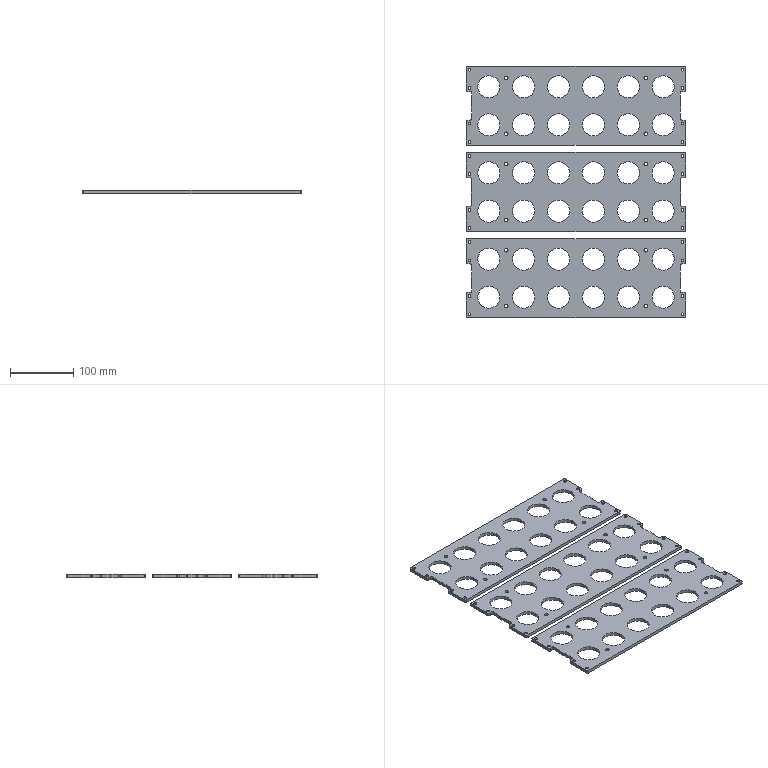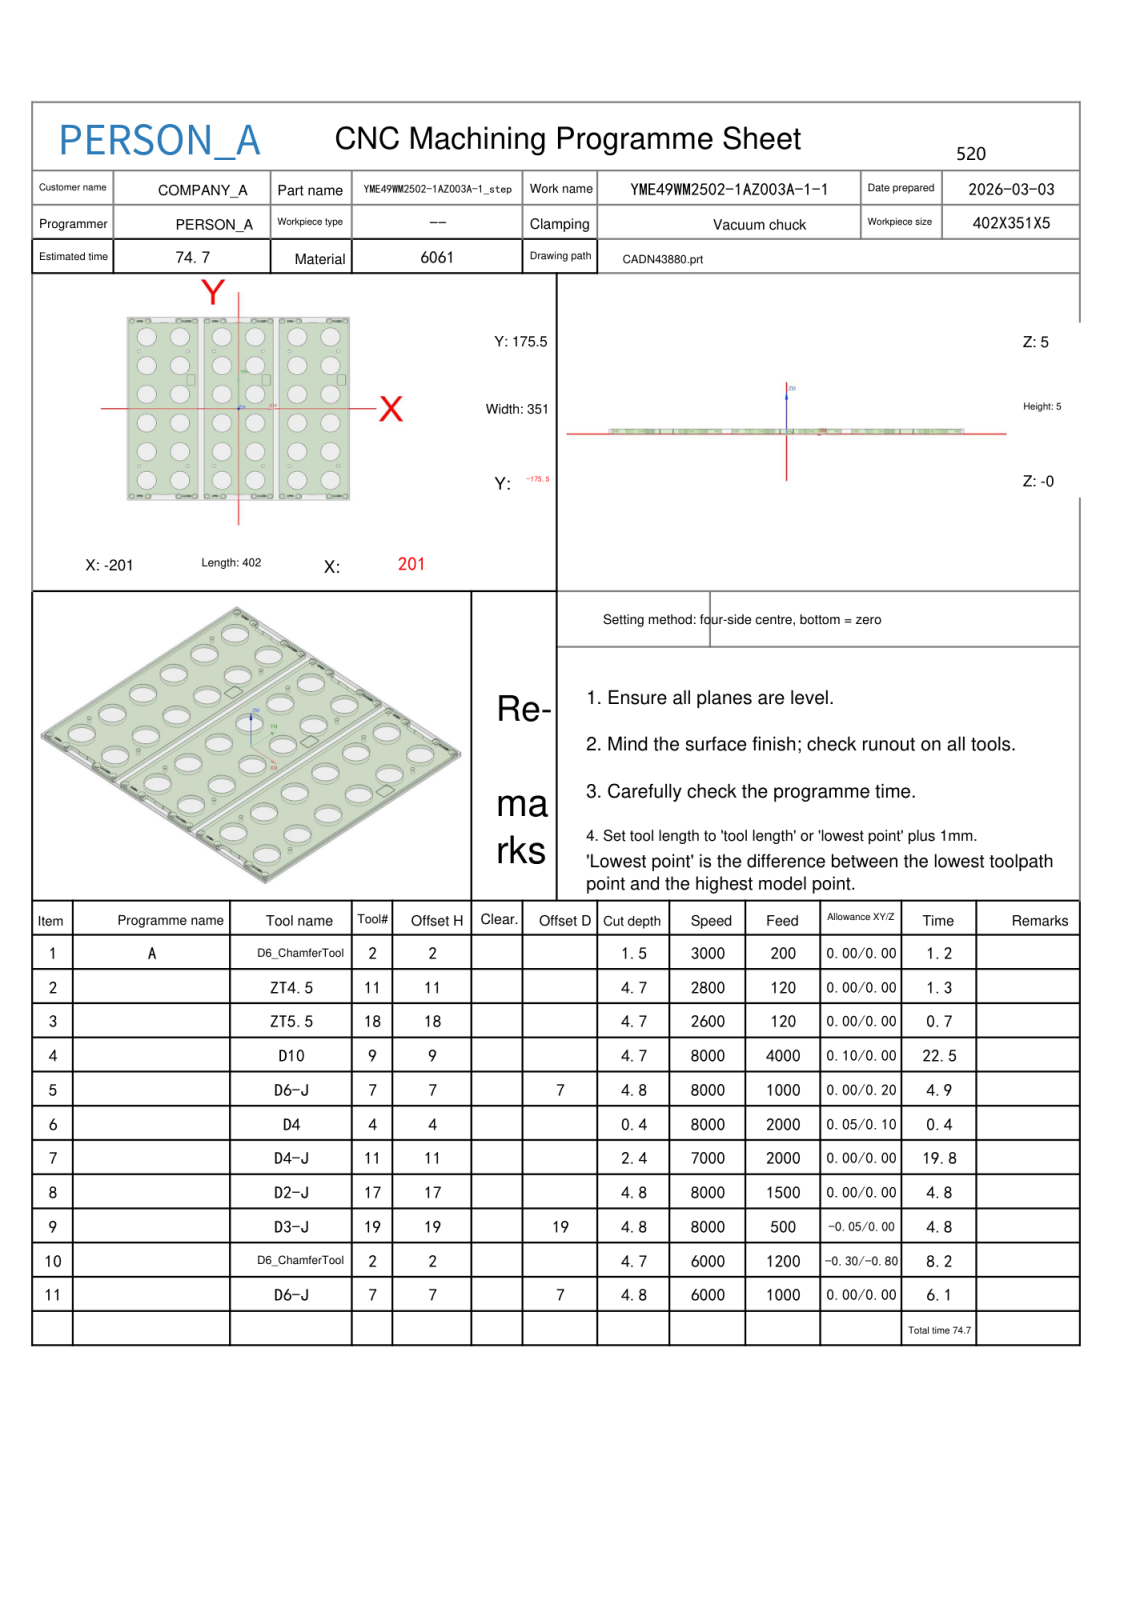NC program | NX | posted by the shop | part box 346 x 397 x 5 mm
Lines 3069 to 4964 of 51232, first 1704 of 1896 lines:
N5 T07 M06
(D6-J  D=6. R=0. H=07 ce=0.00 di=0.20)
G00 G90 G54 X-98.888 Y40.042 M03 S8000
G43 H07 Z35.
M08
Z5.5
G01 X-99.595 Y40.425 Z5.358 F1000.
X-100.545 Y40.854 Z5.174
X-101.524 Y41.213 Z4.991
X-102.526 Y41.5 Z4.807
X-103.547 Y41.715 Z4.623
X-104.58 Y41.855 Z4.439
X-105.62 Y41.92 Z4.255
X-106.38 Z4.121
X-107.419 Y41.855 Z3.938
X-108.45 Y41.715 Z3.754
X-109.469 Y41.502 Z3.571
X-110.47 Y41.215 Z3.387
X-111.447 Y40.857 Z3.204
X-112.396 Y40.429 Z3.02
X-113.312 Y39.935 Z2.837
X-114.189 Y39.375 Z2.653
X-115.024 Y38.753 Z2.469
X-115.812 Y38.073 Z2.286
X-116.549 Y37.338 Z2.102
X-117.231 Y36.552 Z1.919
X-117.855 Y35.718 Z1.735
X-118.417 Y34.842 Z1.552
X-118.914 Y33.928 Z1.368
X-119.344 Y32.98 Z1.185
X-119.704 Y32.003 Z1.001
X-119.993 Y31.003 Z.818
X-120.209 Y29.985 Z.634
X-120.352 Y28.954 Z.451
X-120.419 Y27.915 Z.267
X-120.42 Y27.535 Z.2
X-120.465
G41 D07
X-120.5 Y27.5
G03 X-106. Y13. I14.5 J0.0
X-91.5 Y27.5 I0.0 J14.5
X-106. Y42. I-14.5 J0.0
X-120.5 Y27.5 I0.0 J-14.5
X-120.494 Y27.1 I14.5 J0.0
G01 X-120.484 Y27.048
X-120.444 Y27.01
X-120.392 Y27.003
G40 X-120.342 Y27.004
Z1.2
G00 Z35.
X-98.888 Y95.042
Z5.5
G01 X-99.595 Y95.425 Z5.358
X-100.545 Y95.854 Z5.174
X-101.524 Y96.213 Z4.991
X-102.526 Y96.5 Z4.807
X-103.547 Y96.715 Z4.623
X-104.58 Y96.855 Z4.439
X-105.62 Y96.92 Z4.255
X-106.38 Z4.121
X-107.419 Y96.855 Z3.938
X-108.45 Y96.715 Z3.754
X-109.469 Y96.502 Z3.571
X-110.47 Y96.215 Z3.387
X-111.447 Y95.857 Z3.204
X-112.396 Y95.429 Z3.02
X-113.312 Y94.935 Z2.837
X-114.189 Y94.375 Z2.653
X-115.024 Y93.753 Z2.469
X-115.812 Y93.073 Z2.286
X-116.549 Y92.338 Z2.102
X-117.231 Y91.552 Z1.919
X-117.855 Y90.718 Z1.735
X-118.417 Y89.842 Z1.552
X-118.914 Y88.928 Z1.368
X-119.344 Y87.98 Z1.185
X-119.704 Y87.003 Z1.001
X-119.993 Y86.003 Z.818
X-120.209 Y84.985 Z.634
X-120.352 Y83.954 Z.451
X-120.419 Y82.915 Z.267
X-120.42 Y82.535 Z.2
X-120.465
G41 D07
X-120.5 Y82.5
G03 X-106. Y68. I14.5 J0.0
X-91.5 Y82.5 I0.0 J14.5
X-106. Y97. I-14.5 J0.0
X-120.5 Y82.5 I0.0 J-14.5
X-120.494 Y82.1 I14.5 J0.0
G01 X-120.484 Y82.048
X-120.444 Y82.01
X-120.392 Y82.003
G40 X-120.342 Y82.004
Z1.2
G00 Z35.
X-93.458 Y130.388
Z5.5
G01 X-93.075 Y131.095 Z5.358
X-92.646 Y132.045 Z5.174
X-92.287 Y133.024 Z4.991
X-92. Y134.026 Z4.807
X-91.785 Y135.047 Z4.623
X-91.645 Y136.08 Z4.439
X-91.58 Y137.12 Z4.255
Y137.88 Z4.121
X-91.645 Y138.919 Z3.938
X-91.785 Y139.95 Z3.754
X-91.998 Y140.969 Z3.571
X-92.285 Y141.97 Z3.387
X-92.643 Y142.947 Z3.204
X-93.071 Y143.896 Z3.02
X-93.565 Y144.812 Z2.837
X-94.125 Y145.689 Z2.653
X-94.747 Y146.524 Z2.469
X-95.427 Y147.312 Z2.286
X-96.162 Y148.049 Z2.102
X-96.948 Y148.731 Z1.919
X-97.782 Y149.355 Z1.735
X-98.658 Y149.917 Z1.552
X-99.572 Y150.414 Z1.368
X-100.52 Y150.844 Z1.185
X-101.497 Y151.204 Z1.001
X-102.497 Y151.493 Z.818
X-103.515 Y151.709 Z.634
X-104.546 Y151.852 Z.451
X-105.585 Y151.919 Z.267
X-105.965 Y151.92 Z.2
Y151.965
G41 D07
X-106. Y152.
G03 X-120.5 Y137.5 I0.0 J-14.5
X-106. Y123. I14.5 J0.0
X-91.5 Y137.5 I0.0 J14.5
X-106. Y152. I-14.5 J0.0
X-106.4 Y151.994 I0.0 J-14.5
G01 X-106.452 Y151.984
X-106.49 Y151.944
X-106.497 Y151.892
G40 X-106.496 Y151.842
Z1.2
G00 Z35.
X-153.458 Y130.388
Z5.5
G01 X-153.075 Y131.095 Z5.358
X-152.646 Y132.045 Z5.174
X-152.287 Y133.024 Z4.991
X-152. Y134.026 Z4.807
X-151.785 Y135.047 Z4.623
X-151.645 Y136.08 Z4.439
X-151.58 Y137.12 Z4.255
Y137.88 Z4.121
X-151.645 Y138.919 Z3.938
X-151.785 Y139.95 Z3.754
X-151.998 Y140.969 Z3.571
X-152.285 Y141.97 Z3.387
X-152.643 Y142.947 Z3.204
X-153.071 Y143.896 Z3.02
X-153.565 Y144.812 Z2.837
X-154.125 Y145.689 Z2.653
X-154.747 Y146.524 Z2.469
X-155.427 Y147.312 Z2.286
X-156.162 Y148.049 Z2.102
X-156.948 Y148.731 Z1.919
X-157.782 Y149.355 Z1.735
X-158.658 Y149.917 Z1.552
X-159.572 Y150.414 Z1.368
X-160.52 Y150.844 Z1.185
X-161.497 Y151.204 Z1.001
X-162.497 Y151.493 Z.818
X-163.515 Y151.709 Z.634
X-164.546 Y151.852 Z.451
X-165.585 Y151.919 Z.267
X-165.965 Y151.92 Z.2
Y151.965
G41 D07
X-166. Y152.
G03 X-180.5 Y137.5 I0.0 J-14.5
X-166. Y123. I14.5 J0.0
X-151.5 Y137.5 I0.0 J14.5
X-166. Y152. I-14.5 J0.0
X-166.4 Y151.994 I0.0 J-14.5
G01 X-166.452 Y151.984
X-166.49 Y151.944
X-166.497 Y151.892
G40 X-166.496 Y151.842
Z1.2
G00 Z35.
X-158.888 Y95.042
Z5.5
G01 X-159.595 Y95.425 Z5.358
X-160.545 Y95.854 Z5.174
X-161.524 Y96.213 Z4.991
X-162.526 Y96.5 Z4.807
X-163.547 Y96.715 Z4.623
X-164.58 Y96.855 Z4.439
X-165.62 Y96.92 Z4.255
X-166.38 Z4.121
X-167.419 Y96.855 Z3.938
X-168.45 Y96.715 Z3.754
X-169.469 Y96.502 Z3.571
X-170.47 Y96.215 Z3.387
X-171.447 Y95.857 Z3.204
X-172.396 Y95.429 Z3.02
X-173.312 Y94.935 Z2.837
X-174.189 Y94.375 Z2.653
X-175.024 Y93.753 Z2.469
X-175.812 Y93.073 Z2.286
X-176.549 Y92.338 Z2.102
X-177.231 Y91.552 Z1.919
X-177.855 Y90.718 Z1.735
X-178.417 Y89.842 Z1.552
X-178.914 Y88.928 Z1.368
X-179.344 Y87.98 Z1.185
X-179.704 Y87.003 Z1.001
X-179.993 Y86.003 Z.818
X-180.209 Y84.985 Z.634
X-180.352 Y83.954 Z.451
X-180.419 Y82.915 Z.267
X-180.42 Y82.535 Z.2
X-180.465
G41 D07
X-180.5 Y82.5
G03 X-166. Y68. I14.5 J0.0
X-151.5 Y82.5 I0.0 J14.5
X-166. Y97. I-14.5 J0.0
X-180.5 Y82.5 I0.0 J-14.5
X-180.494 Y82.1 I14.5 J0.0
G01 X-180.484 Y82.048
X-180.444 Y82.01
X-180.392 Y82.003
G40 X-180.342 Y82.004
Z1.2
G00 Z35.
X-158.888 Y40.042
Z5.5
G01 X-159.595 Y40.425 Z5.358
X-160.545 Y40.854 Z5.174
X-161.524 Y41.213 Z4.991
X-162.526 Y41.5 Z4.807
X-163.547 Y41.715 Z4.623
X-164.58 Y41.855 Z4.439
X-165.62 Y41.92 Z4.255
X-166.38 Z4.121
X-167.419 Y41.855 Z3.938
X-168.45 Y41.715 Z3.754
X-169.469 Y41.502 Z3.571
X-170.47 Y41.215 Z3.387
X-171.447 Y40.857 Z3.204
X-172.396 Y40.429 Z3.02
X-173.312 Y39.935 Z2.837
X-174.189 Y39.375 Z2.653
X-175.024 Y38.753 Z2.469
X-175.812 Y38.073 Z2.286
X-176.549 Y37.338 Z2.102
X-177.231 Y36.552 Z1.919
X-177.855 Y35.718 Z1.735
X-178.417 Y34.842 Z1.552
X-178.914 Y33.928 Z1.368
X-179.344 Y32.98 Z1.185
X-179.704 Y32.003 Z1.001
X-179.993 Y31.003 Z.818
X-180.209 Y29.985 Z.634
X-180.352 Y28.954 Z.451
X-180.419 Y27.915 Z.267
X-180.42 Y27.535 Z.2
X-180.465
G41 D07
X-180.5 Y27.5
G03 X-166. Y13. I14.5 J0.0
X-151.5 Y27.5 I0.0 J14.5
X-166. Y42. I-14.5 J0.0
X-180.5 Y27.5 I0.0 J-14.5
X-180.494 Y27.1 I14.5 J0.0
G01 X-180.484 Y27.048
X-180.444 Y27.01
X-180.392 Y27.003
G40 X-180.342 Y27.004
Z1.2
G00 Z35.
X-158.888 Y-14.958
Z5.5
G01 X-159.595 Y-14.575 Z5.358
X-160.545 Y-14.146 Z5.174
X-161.524 Y-13.787 Z4.991
X-162.526 Y-13.5 Z4.807
X-163.547 Y-13.285 Z4.623
X-164.58 Y-13.145 Z4.439
X-165.62 Y-13.08 Z4.255
X-166.38 Z4.121
X-167.419 Y-13.145 Z3.938
X-168.45 Y-13.285 Z3.754
X-169.469 Y-13.498 Z3.571
X-170.47 Y-13.785 Z3.387
X-171.447 Y-14.143 Z3.204
X-172.396 Y-14.571 Z3.02
X-173.312 Y-15.065 Z2.837
X-174.189 Y-15.625 Z2.653
X-175.024 Y-16.247 Z2.469
X-175.812 Y-16.927 Z2.286
X-176.549 Y-17.662 Z2.102
X-177.231 Y-18.448 Z1.919
X-177.855 Y-19.282 Z1.735
X-178.417 Y-20.158 Z1.552
X-178.914 Y-21.072 Z1.368
X-179.344 Y-22.02 Z1.185
X-179.704 Y-22.997 Z1.001
X-179.993 Y-23.997 Z.818
X-180.209 Y-25.015 Z.634
X-180.352 Y-26.046 Z.451
X-180.419 Y-27.085 Z.267
X-180.42 Y-27.465 Z.2
X-180.465
G41 D07
X-180.5 Y-27.5
G03 X-166. Y-42. I14.5 J0.0
X-151.5 Y-27.5 I0.0 J14.5
X-166. Y-13. I-14.5 J0.0
X-180.5 Y-27.5 I0.0 J-14.5
X-180.494 Y-27.9 I14.5 J0.0
G01 X-180.484 Y-27.952
X-180.444 Y-27.99
X-180.392 Y-27.997
G40 X-180.342 Y-27.996
Z1.2
G00 Z35.
X-158.888 Y-69.958
Z5.5
G01 X-159.595 Y-69.575 Z5.358
X-160.545 Y-69.146 Z5.174
X-161.524 Y-68.787 Z4.991
X-162.526 Y-68.5 Z4.807
X-163.547 Y-68.285 Z4.623
X-164.58 Y-68.145 Z4.439
X-165.62 Y-68.08 Z4.255
X-166.38 Z4.121
X-167.419 Y-68.145 Z3.938
X-168.45 Y-68.285 Z3.754
X-169.469 Y-68.498 Z3.571
X-170.47 Y-68.785 Z3.387
X-171.447 Y-69.143 Z3.204
X-172.396 Y-69.571 Z3.02
X-173.312 Y-70.065 Z2.837
X-174.189 Y-70.625 Z2.653
X-175.024 Y-71.247 Z2.469
X-175.812 Y-71.927 Z2.286
X-176.549 Y-72.662 Z2.102
X-177.231 Y-73.448 Z1.919
X-177.855 Y-74.282 Z1.735
X-178.417 Y-75.158 Z1.552
X-178.914 Y-76.072 Z1.368
X-179.344 Y-77.02 Z1.185
X-179.704 Y-77.997 Z1.001
X-179.993 Y-78.997 Z.818
X-180.209 Y-80.015 Z.634
X-180.352 Y-81.046 Z.451
X-180.419 Y-82.085 Z.267
X-180.42 Y-82.465 Z.2
X-180.465
G41 D07
X-180.5 Y-82.5
G03 X-166. Y-97. I14.5 J0.0
X-151.5 Y-82.5 I0.0 J14.5
X-166. Y-68. I-14.5 J0.0
X-180.5 Y-82.5 I0.0 J-14.5
X-180.494 Y-82.9 I14.5 J0.0
G01 X-180.484 Y-82.952
X-180.444 Y-82.99
X-180.392 Y-82.997
G40 X-180.342 Y-82.996
Z1.2
G00 Z35.
X-158.888 Y-124.958
Z5.5
G01 X-159.595 Y-124.575 Z5.358
X-160.545 Y-124.146 Z5.174
X-161.524 Y-123.787 Z4.991
X-162.526 Y-123.5 Z4.807
X-163.547 Y-123.285 Z4.623
X-164.58 Y-123.145 Z4.439
X-165.62 Y-123.08 Z4.255
X-166.38 Z4.121
X-167.419 Y-123.145 Z3.938
X-168.45 Y-123.285 Z3.754
X-169.469 Y-123.498 Z3.571
X-170.47 Y-123.785 Z3.387
X-171.447 Y-124.143 Z3.204
X-172.396 Y-124.571 Z3.02
X-173.312 Y-125.065 Z2.837
X-174.189 Y-125.625 Z2.653
X-175.024 Y-126.247 Z2.469
X-175.812 Y-126.927 Z2.286
X-176.549 Y-127.662 Z2.102
X-177.231 Y-128.448 Z1.919
X-177.855 Y-129.282 Z1.735
X-178.417 Y-130.158 Z1.552
X-178.914 Y-131.072 Z1.368
X-179.344 Y-132.02 Z1.185
X-179.704 Y-132.997 Z1.001
X-179.993 Y-133.997 Z.818
X-180.209 Y-135.015 Z.634
X-180.352 Y-136.046 Z.451
X-180.419 Y-137.085 Z.267
X-180.42 Y-137.465 Z.2
X-180.465
G41 D07
X-180.5 Y-137.5
G03 X-166. Y-152. I14.5 J0.0
X-151.5 Y-137.5 I0.0 J14.5
X-166. Y-123. I-14.5 J0.0
X-180.5 Y-137.5 I0.0 J-14.5
X-180.494 Y-137.9 I14.5 J0.0
G01 X-180.484 Y-137.952
X-180.444 Y-137.99
X-180.392 Y-137.997
G40 X-180.342 Y-137.996
Z1.2
G00 Z35.
X-118.542 Y-130.388
Z5.5
G01 X-118.925 Y-131.095 Z5.358
X-119.354 Y-132.045 Z5.174
X-119.713 Y-133.024 Z4.991
X-120. Y-134.026 Z4.807
X-120.215 Y-135.047 Z4.623
X-120.355 Y-136.08 Z4.439
X-120.42 Y-137.12 Z4.255
Y-137.88 Z4.121
X-120.355 Y-138.919 Z3.938
X-120.215 Y-139.95 Z3.754
X-120.002 Y-140.969 Z3.571
X-119.715 Y-141.97 Z3.387
X-119.357 Y-142.947 Z3.204
X-118.929 Y-143.896 Z3.02
X-118.435 Y-144.812 Z2.837
X-117.875 Y-145.689 Z2.653
X-117.253 Y-146.524 Z2.469
X-116.573 Y-147.312 Z2.286
X-115.838 Y-148.049 Z2.102
X-115.052 Y-148.731 Z1.919
X-114.218 Y-149.355 Z1.735
X-113.342 Y-149.917 Z1.552
X-112.428 Y-150.414 Z1.368
X-111.48 Y-150.844 Z1.185
X-110.503 Y-151.204 Z1.001
X-109.503 Y-151.493 Z.818
X-108.485 Y-151.709 Z.634
X-107.454 Y-151.852 Z.451
X-106.415 Y-151.919 Z.267
X-106.035 Y-151.92 Z.2
Y-151.965
G41 D07
X-106. Y-152.
G03 X-91.5 Y-137.5 I0.0 J14.5
X-106. Y-123. I-14.5 J0.0
X-120.5 Y-137.5 I0.0 J-14.5
X-106. Y-152. I14.5 J0.0
X-105.6 Y-151.994 I0.0 J14.5
G01 X-105.548 Y-151.984
X-105.51 Y-151.944
X-105.503 Y-151.892
G40 X-105.504 Y-151.842
Z1.2
G00 Z35.
X-118.542 Y-75.388
Z5.5
G01 X-118.925 Y-76.095 Z5.358
X-119.354 Y-77.045 Z5.174
X-119.713 Y-78.024 Z4.991
X-120. Y-79.026 Z4.807
X-120.215 Y-80.047 Z4.623
X-120.355 Y-81.08 Z4.439
X-120.42 Y-82.12 Z4.255
Y-82.88 Z4.121
X-120.355 Y-83.919 Z3.938
X-120.215 Y-84.95 Z3.754
X-120.002 Y-85.969 Z3.571
X-119.715 Y-86.97 Z3.387
X-119.357 Y-87.947 Z3.204
X-118.929 Y-88.896 Z3.02
X-118.435 Y-89.812 Z2.837
X-117.875 Y-90.689 Z2.653
X-117.253 Y-91.524 Z2.469
X-116.573 Y-92.312 Z2.286
X-115.838 Y-93.049 Z2.102
X-115.052 Y-93.731 Z1.919
X-114.218 Y-94.355 Z1.735
X-113.342 Y-94.917 Z1.552
X-112.428 Y-95.414 Z1.368
X-111.48 Y-95.844 Z1.185
X-110.503 Y-96.204 Z1.001
X-109.503 Y-96.493 Z.818
X-108.485 Y-96.709 Z.634
X-107.454 Y-96.852 Z.451
X-106.415 Y-96.919 Z.267
X-106.035 Y-96.92 Z.2
Y-96.965
G41 D07
X-106. Y-97.
G03 X-91.5 Y-82.5 I0.0 J14.5
X-106. Y-68. I-14.5 J0.0
X-120.5 Y-82.5 I0.0 J-14.5
X-106. Y-97. I14.5 J0.0
X-105.6 Y-96.994 I0.0 J14.5
G01 X-105.548 Y-96.984
X-105.51 Y-96.944
X-105.503 Y-96.892
G40 X-105.504 Y-96.842
Z1.2
G00 Z35.
X-98.888 Y-14.958
Z5.5
G01 X-99.595 Y-14.575 Z5.358
X-100.545 Y-14.146 Z5.174
X-101.524 Y-13.787 Z4.991
X-102.526 Y-13.5 Z4.807
X-103.547 Y-13.285 Z4.623
X-104.58 Y-13.145 Z4.439
X-105.62 Y-13.08 Z4.255
X-106.38 Z4.121
X-107.419 Y-13.145 Z3.938
X-108.45 Y-13.285 Z3.754
X-109.469 Y-13.498 Z3.571
X-110.47 Y-13.785 Z3.387
X-111.447 Y-14.143 Z3.204
X-112.396 Y-14.571 Z3.02
X-113.312 Y-15.065 Z2.837
X-114.189 Y-15.625 Z2.653
X-115.024 Y-16.247 Z2.469
X-115.812 Y-16.927 Z2.286
X-116.549 Y-17.662 Z2.102
X-117.231 Y-18.448 Z1.919
X-117.855 Y-19.282 Z1.735
X-118.417 Y-20.158 Z1.552
X-118.914 Y-21.072 Z1.368
X-119.344 Y-22.02 Z1.185
X-119.704 Y-22.997 Z1.001
X-119.993 Y-23.997 Z.818
X-120.209 Y-25.015 Z.634
X-120.352 Y-26.046 Z.451
X-120.419 Y-27.085 Z.267
X-120.42 Y-27.465 Z.2
X-120.465
G41 D07
X-120.5 Y-27.5
G03 X-106. Y-42. I14.5 J0.0
X-91.5 Y-27.5 I0.0 J14.5
X-106. Y-13. I-14.5 J0.0
X-120.5 Y-27.5 I0.0 J-14.5
X-120.494 Y-27.9 I14.5 J0.0
G01 X-120.484 Y-27.952
X-120.444 Y-27.99
X-120.392 Y-27.997
G40 X-120.342 Y-27.996
Z1.2
G00 Z35.
X-42.542 Y-20.388
Z5.5
G01 X-42.925 Y-21.095 Z5.358
X-43.354 Y-22.045 Z5.174
X-43.713 Y-23.024 Z4.991
X-44. Y-24.026 Z4.807
X-44.215 Y-25.047 Z4.623
X-44.355 Y-26.08 Z4.439
X-44.42 Y-27.12 Z4.255
Y-27.88 Z4.121
X-44.355 Y-28.919 Z3.938
X-44.215 Y-29.95 Z3.754
X-44.002 Y-30.969 Z3.571
X-43.715 Y-31.97 Z3.387
X-43.357 Y-32.947 Z3.204
X-42.929 Y-33.896 Z3.02
X-42.435 Y-34.812 Z2.837
X-41.875 Y-35.689 Z2.653
X-41.253 Y-36.524 Z2.469
X-40.573 Y-37.312 Z2.286
X-39.838 Y-38.049 Z2.102
X-39.052 Y-38.731 Z1.919
X-38.218 Y-39.355 Z1.735
X-37.342 Y-39.917 Z1.552
X-36.428 Y-40.414 Z1.368
X-35.48 Y-40.844 Z1.185
X-34.503 Y-41.204 Z1.001
X-33.503 Y-41.493 Z.818
X-32.485 Y-41.709 Z.634
X-31.454 Y-41.852 Z.451
X-30.415 Y-41.919 Z.267
X-30.035 Y-41.92 Z.2
Y-41.965
G41 D07
X-30. Y-42.
G03 X-15.5 Y-27.5 I0.0 J14.5
X-30. Y-13. I-14.5 J0.0
X-44.5 Y-27.5 I0.0 J-14.5
X-30. Y-42. I14.5 J0.0
X-29.6 Y-41.994 I0.0 J14.5
G01 X-29.548 Y-41.984
X-29.51 Y-41.944
X-29.503 Y-41.892
G40 X-29.504 Y-41.842
Z1.2
G00 Z35.
X-17.458 Y20.388
Z5.5
G01 X-17.075 Y21.095 Z5.358
X-16.646 Y22.045 Z5.174
X-16.287 Y23.024 Z4.991
X-16. Y24.026 Z4.807
X-15.785 Y25.047 Z4.623
X-15.645 Y26.08 Z4.439
X-15.58 Y27.12 Z4.255
Y27.88 Z4.121
X-15.645 Y28.919 Z3.938
X-15.785 Y29.95 Z3.754
X-15.998 Y30.969 Z3.571
X-16.285 Y31.97 Z3.387
X-16.643 Y32.947 Z3.204
X-17.071 Y33.896 Z3.02
X-17.565 Y34.812 Z2.837
X-18.125 Y35.689 Z2.653
X-18.747 Y36.524 Z2.469
X-19.427 Y37.312 Z2.286
X-20.162 Y38.049 Z2.102
X-20.948 Y38.731 Z1.919
X-21.782 Y39.355 Z1.735
X-22.658 Y39.917 Z1.552
X-23.572 Y40.414 Z1.368
X-24.52 Y40.844 Z1.185
X-25.497 Y41.204 Z1.001
X-26.497 Y41.493 Z.818
X-27.515 Y41.709 Z.634
X-28.546 Y41.852 Z.451
X-29.585 Y41.919 Z.267
X-29.965 Y41.92 Z.2
Y41.965
G41 D07
X-30. Y42.
G03 X-44.5 Y27.5 I0.0 J-14.5
X-30. Y13. I14.5 J0.0
X-15.5 Y27.5 I0.0 J14.5
X-30. Y42. I-14.5 J0.0
X-30.4 Y41.994 I0.0 J-14.5
G01 X-30.452 Y41.984
X-30.49 Y41.944
X-30.497 Y41.892
G40 X-30.496 Y41.842
Z1.2
G00 Z35.
X-17.458 Y75.388
Z5.5
G01 X-17.075 Y76.095 Z5.358
X-16.646 Y77.045 Z5.174
X-16.287 Y78.024 Z4.991
X-16. Y79.026 Z4.807
X-15.785 Y80.047 Z4.623
X-15.645 Y81.08 Z4.439
X-15.58 Y82.12 Z4.255
Y82.88 Z4.121
X-15.645 Y83.919 Z3.938
X-15.785 Y84.95 Z3.754
X-15.998 Y85.969 Z3.571
X-16.285 Y86.97 Z3.387
X-16.643 Y87.947 Z3.204
X-17.071 Y88.896 Z3.02
X-17.565 Y89.812 Z2.837
X-18.125 Y90.689 Z2.653
X-18.747 Y91.524 Z2.469
X-19.427 Y92.312 Z2.286
X-20.162 Y93.049 Z2.102
X-20.948 Y93.731 Z1.919
X-21.782 Y94.355 Z1.735
X-22.658 Y94.917 Z1.552
X-23.572 Y95.414 Z1.368
X-24.52 Y95.844 Z1.185
X-25.497 Y96.204 Z1.001
X-26.497 Y96.493 Z.818
X-27.515 Y96.709 Z.634
X-28.546 Y96.852 Z.451
X-29.585 Y96.919 Z.267
X-29.965 Y96.92 Z.2
Y96.965
G41 D07
X-30. Y97.
G03 X-44.5 Y82.5 I0.0 J-14.5
X-30. Y68. I14.5 J0.0
X-15.5 Y82.5 I0.0 J14.5
X-30. Y97. I-14.5 J0.0
X-30.4 Y96.994 I0.0 J-14.5
G01 X-30.452 Y96.984
X-30.49 Y96.944
X-30.497 Y96.892
G40 X-30.496 Y96.842
Z1.2
G00 Z35.
X-17.458 Y130.388
Z5.5
G01 X-17.075 Y131.095 Z5.358
X-16.646 Y132.045 Z5.174
X-16.287 Y133.024 Z4.991
X-16. Y134.026 Z4.807
X-15.785 Y135.047 Z4.623
X-15.645 Y136.08 Z4.439
X-15.58 Y137.12 Z4.255
Y137.88 Z4.121
X-15.645 Y138.919 Z3.938
X-15.785 Y139.95 Z3.754
X-15.998 Y140.969 Z3.571
X-16.285 Y141.97 Z3.387
X-16.643 Y142.947 Z3.204
X-17.071 Y143.896 Z3.02
X-17.565 Y144.812 Z2.837
X-18.125 Y145.689 Z2.653
X-18.747 Y146.524 Z2.469
X-19.427 Y147.312 Z2.286
X-20.162 Y148.049 Z2.102
X-20.948 Y148.731 Z1.919
X-21.782 Y149.355 Z1.735
X-22.658 Y149.917 Z1.552
X-23.572 Y150.414 Z1.368
X-24.52 Y150.844 Z1.185
X-25.497 Y151.204 Z1.001
X-26.497 Y151.493 Z.818
X-27.515 Y151.709 Z.634
X-28.546 Y151.852 Z.451
X-29.585 Y151.919 Z.267
X-29.965 Y151.92 Z.2
Y151.965
G41 D07
X-30. Y152.
G03 X-44.5 Y137.5 I0.0 J-14.5
X-30. Y123. I14.5 J0.0
X-15.5 Y137.5 I0.0 J14.5
X-30. Y152. I-14.5 J0.0
X-30.4 Y151.994 I0.0 J-14.5
G01 X-30.452 Y151.984
X-30.49 Y151.944
X-30.497 Y151.892
G40 X-30.496 Y151.842
Z1.2
G00 Z35.
X42.542 Y130.388
Z5.5
G01 X42.925 Y131.095 Z5.358
X43.354 Y132.045 Z5.174
X43.713 Y133.024 Z4.991
X44. Y134.026 Z4.807
X44.215 Y135.047 Z4.623
X44.355 Y136.08 Z4.439
X44.42 Y137.12 Z4.255
Y137.88 Z4.121
X44.355 Y138.919 Z3.938
X44.215 Y139.95 Z3.754
X44.002 Y140.969 Z3.571
X43.715 Y141.97 Z3.387
X43.357 Y142.947 Z3.204
X42.929 Y143.896 Z3.02
X42.435 Y144.812 Z2.837
X41.875 Y145.689 Z2.653
X41.253 Y146.524 Z2.469
X40.573 Y147.312 Z2.286
X39.838 Y148.049 Z2.102
X39.052 Y148.731 Z1.919
X38.218 Y149.355 Z1.735
X37.342 Y149.917 Z1.552
X36.428 Y150.414 Z1.368
X35.48 Y150.844 Z1.185
X34.503 Y151.204 Z1.001
X33.503 Y151.493 Z.818
X32.485 Y151.709 Z.634
X31.454 Y151.852 Z.451
X30.415 Y151.919 Z.267
X30.035 Y151.92 Z.2
Y151.965
G41 D07
X30. Y152.
G03 X15.5 Y137.5 I0.0 J-14.5
X30. Y123. I14.5 J0.0
X44.5 Y137.5 I0.0 J14.5
X30. Y152. I-14.5 J0.0
X29.6 Y151.994 I0.0 J-14.5
G01 X29.548 Y151.984
X29.51 Y151.944
X29.503 Y151.892
G40 X29.504 Y151.842
Z1.2
G00 Z35.
X42.542 Y75.388
Z5.5
G01 X42.925 Y76.095 Z5.358
X43.354 Y77.045 Z5.174
X43.713 Y78.024 Z4.991
X44. Y79.026 Z4.807
X44.215 Y80.047 Z4.623
X44.355 Y81.08 Z4.439
X44.42 Y82.12 Z4.255
Y82.88 Z4.121
X44.355 Y83.919 Z3.938
X44.215 Y84.95 Z3.754
X44.002 Y85.969 Z3.571
X43.715 Y86.97 Z3.387
X43.357 Y87.947 Z3.204
X42.929 Y88.896 Z3.02
X42.435 Y89.812 Z2.837
X41.875 Y90.689 Z2.653
X41.253 Y91.524 Z2.469
X40.573 Y92.312 Z2.286
X39.838 Y93.049 Z2.102
X39.052 Y93.731 Z1.919
X38.218 Y94.355 Z1.735
X37.342 Y94.917 Z1.552
X36.428 Y95.414 Z1.368
X35.48 Y95.844 Z1.185
X34.503 Y96.204 Z1.001
X33.503 Y96.493 Z.818
X32.485 Y96.709 Z.634
X31.454 Y96.852 Z.451
X30.415 Y96.919 Z.267
X30.035 Y96.92 Z.2
Y96.965
G41 D07
X30. Y97.
G03 X15.5 Y82.5 I0.0 J-14.5
X30. Y68. I14.5 J0.0
X44.5 Y82.5 I0.0 J14.5
X30. Y97. I-14.5 J0.0
X29.6 Y96.994 I0.0 J-14.5
G01 X29.548 Y96.984
X29.51 Y96.944
X29.503 Y96.892
G40 X29.504 Y96.842
Z1.2
G00 Z35.
X42.542 Y20.388
Z5.5
G01 X42.925 Y21.095 Z5.358
X43.354 Y22.045 Z5.174
X43.713 Y23.024 Z4.991
X44. Y24.026 Z4.807
X44.215 Y25.047 Z4.623
X44.355 Y26.08 Z4.439
X44.42 Y27.12 Z4.255
Y27.88 Z4.121
X44.355 Y28.919 Z3.938
X44.215 Y29.95 Z3.754
X44.002 Y30.969 Z3.571
X43.715 Y31.97 Z3.387
X43.357 Y32.947 Z3.204
X42.929 Y33.896 Z3.02
X42.435 Y34.812 Z2.837
X41.875 Y35.689 Z2.653
X41.253 Y36.524 Z2.469
X40.573 Y37.312 Z2.286
X39.838 Y38.049 Z2.102
X39.052 Y38.731 Z1.919
X38.218 Y39.355 Z1.735
X37.342 Y39.917 Z1.552
X36.428 Y40.414 Z1.368
X35.48 Y40.844 Z1.185
X34.503 Y41.204 Z1.001
X33.503 Y41.493 Z.818
X32.485 Y41.709 Z.634
X31.454 Y41.852 Z.451
X30.415 Y41.919 Z.267
X30.035 Y41.92 Z.2
Y41.965
G41 D07
X30. Y42.
G03 X15.5 Y27.5 I0.0 J-14.5
X30. Y13. I14.5 J0.0
X44.5 Y27.5 I0.0 J14.5
X30. Y42. I-14.5 J0.0
X29.6 Y41.994 I0.0 J-14.5
G01 X29.548 Y41.984
X29.51 Y41.944
X29.503 Y41.892
G40 X29.504 Y41.842
Z1.2
G00 Z35.
X17.458 Y-20.388
Z5.5
G01 X17.075 Y-21.095 Z5.358
X16.646 Y-22.045 Z5.174
X16.287 Y-23.024 Z4.991
X16. Y-24.026 Z4.807
X15.785 Y-25.047 Z4.623
X15.645 Y-26.08 Z4.439
X15.58 Y-27.12 Z4.255
Y-27.88 Z4.121
X15.645 Y-28.919 Z3.938
X15.785 Y-29.95 Z3.754
X15.998 Y-30.969 Z3.571
X16.285 Y-31.97 Z3.387
X16.643 Y-32.947 Z3.204
X17.071 Y-33.896 Z3.02
X17.565 Y-34.812 Z2.837
X18.125 Y-35.689 Z2.653
X18.747 Y-36.524 Z2.469
X19.427 Y-37.312 Z2.286
X20.162 Y-38.049 Z2.102
X20.948 Y-38.731 Z1.919
X21.782 Y-39.355 Z1.735
X22.658 Y-39.917 Z1.552
X23.572 Y-40.414 Z1.368
X24.52 Y-40.844 Z1.185
X25.497 Y-41.204 Z1.001
X26.497 Y-41.493 Z.818
X27.515 Y-41.709 Z.634
X28.546 Y-41.852 Z.451
X29.585 Y-41.919 Z.267
X29.965 Y-41.92 Z.2
Y-41.965
G41 D07
X30. Y-42.
G03 X44.5 Y-27.5 I0.0 J14.5
X30. Y-13. I-14.5 J0.0
X15.5 Y-27.5 I0.0 J-14.5
X30. Y-42. I14.5 J0.0
X30.4 Y-41.994 I0.0 J14.5
G01 X30.452 Y-41.984
X30.49 Y-41.944
X30.497 Y-41.892
G40 X30.496 Y-41.842
Z1.2
G00 Z35.
X17.458 Y-75.388
Z5.5
G01 X17.075 Y-76.095 Z5.358
X16.646 Y-77.045 Z5.174
X16.287 Y-78.024 Z4.991
X16. Y-79.026 Z4.807
X15.785 Y-80.047 Z4.623
X15.645 Y-81.08 Z4.439
X15.58 Y-82.12 Z4.255
Y-82.88 Z4.121
X15.645 Y-83.919 Z3.938
X15.785 Y-84.95 Z3.754
X15.998 Y-85.969 Z3.571
X16.285 Y-86.97 Z3.387
X16.643 Y-87.947 Z3.204
X17.071 Y-88.896 Z3.02
X17.565 Y-89.812 Z2.837
X18.125 Y-90.689 Z2.653
X18.747 Y-91.524 Z2.469
X19.427 Y-92.312 Z2.286
X20.162 Y-93.049 Z2.102
X20.948 Y-93.731 Z1.919
X21.782 Y-94.355 Z1.735
X22.658 Y-94.917 Z1.552
X23.572 Y-95.414 Z1.368
X24.52 Y-95.844 Z1.185
X25.497 Y-96.204 Z1.001
X26.497 Y-96.493 Z.818
X27.515 Y-96.709 Z.634
X28.546 Y-96.852 Z.451
X29.585 Y-96.919 Z.267
X29.965 Y-96.92 Z.2
Y-96.965
G41 D07
X30. Y-97.
G03 X44.5 Y-82.5 I0.0 J14.5
X30. Y-68. I-14.5 J0.0
X15.5 Y-82.5 I0.0 J-14.5
X30. Y-97. I14.5 J0.0
X30.4 Y-96.994 I0.0 J14.5
G01 X30.452 Y-96.984
X30.49 Y-96.944
X30.497 Y-96.892
G40 X30.496 Y-96.842
Z1.2
G00 Z35.
X-42.542 Y-75.388
Z5.5
G01 X-42.925 Y-76.095 Z5.358
X-43.354 Y-77.045 Z5.174
X-43.713 Y-78.024 Z4.991
X-44. Y-79.026 Z4.807
X-44.215 Y-80.047 Z4.623
X-44.355 Y-81.08 Z4.439
X-44.42 Y-82.12 Z4.255
Y-82.88 Z4.121
X-44.355 Y-83.919 Z3.938
X-44.215 Y-84.95 Z3.754
X-44.002 Y-85.969 Z3.571
X-43.715 Y-86.97 Z3.387
X-43.357 Y-87.947 Z3.204
X-42.929 Y-88.896 Z3.02
X-42.435 Y-89.812 Z2.837
X-41.875 Y-90.689 Z2.653
X-41.253 Y-91.524 Z2.469
X-40.573 Y-92.312 Z2.286
X-39.838 Y-93.049 Z2.102
X-39.052 Y-93.731 Z1.919
X-38.218 Y-94.355 Z1.735
X-37.342 Y-94.917 Z1.552
X-36.428 Y-95.414 Z1.368
X-35.48 Y-95.844 Z1.185
X-34.503 Y-96.204 Z1.001
X-33.503 Y-96.493 Z.818
X-32.485 Y-96.709 Z.634
X-31.454 Y-96.852 Z.451
X-30.415 Y-96.919 Z.267
X-30.035 Y-96.92 Z.2
Y-96.965
G41 D07
X-30. Y-97.
G03 X-15.5 Y-82.5 I0.0 J14.5
X-30. Y-68. I-14.5 J0.0
X-44.5 Y-82.5 I0.0 J-14.5
X-30. Y-97. I14.5 J0.0
X-29.6 Y-96.994 I0.0 J14.5
G01 X-29.548 Y-96.984
X-29.51 Y-96.944
X-29.503 Y-96.892
G40 X-29.504 Y-96.842
Z1.2
G00 Z35.
X-42.542 Y-130.388
Z5.5
G01 X-42.925 Y-131.095 Z5.358
X-43.354 Y-132.045 Z5.174
X-43.713 Y-133.024 Z4.991
X-44. Y-134.026 Z4.807
X-44.215 Y-135.047 Z4.623
X-44.355 Y-136.08 Z4.439
X-44.42 Y-137.12 Z4.255
Y-137.88 Z4.121
X-44.355 Y-138.919 Z3.938
X-44.215 Y-139.95 Z3.754
X-44.002 Y-140.969 Z3.571
X-43.715 Y-141.97 Z3.387
X-43.357 Y-142.947 Z3.204
X-42.929 Y-143.896 Z3.02
X-42.435 Y-144.812 Z2.837
X-41.875 Y-145.689 Z2.653
X-41.253 Y-146.524 Z2.469
X-40.573 Y-147.312 Z2.286
X-39.838 Y-148.049 Z2.102
X-39.052 Y-148.731 Z1.919
X-38.218 Y-149.355 Z1.735
X-37.342 Y-149.917 Z1.552
X-36.428 Y-150.414 Z1.368
X-35.48 Y-150.844 Z1.185
X-34.503 Y-151.204 Z1.001
X-33.503 Y-151.493 Z.818
X-32.485 Y-151.709 Z.634
X-31.454 Y-151.852 Z.451
X-30.415 Y-151.919 Z.267
X-30.035 Y-151.92 Z.2
Y-151.965
G41 D07
X-30. Y-152.
G03 X-15.5 Y-137.5 I0.0 J14.5
X-30. Y-123. I-14.5 J0.0
X-44.5 Y-137.5 I0.0 J-14.5
X-30. Y-152. I14.5 J0.0
X-29.6 Y-151.994 I0.0 J14.5
G01 X-29.548 Y-151.984
X-29.51 Y-151.944
X-29.503 Y-151.892
G40 X-29.504 Y-151.842
Z1.2
G00 Z35.
X17.458 Y-130.388
Z5.5
G01 X17.075 Y-131.095 Z5.358
X16.646 Y-132.045 Z5.174
X16.287 Y-133.024 Z4.991
X16. Y-134.026 Z4.807
X15.785 Y-135.047 Z4.623
X15.645 Y-136.08 Z4.439
X15.58 Y-137.12 Z4.255
Y-137.88 Z4.121
X15.645 Y-138.919 Z3.938
X15.785 Y-139.95 Z3.754
X15.998 Y-140.969 Z3.571
X16.285 Y-141.97 Z3.387
X16.643 Y-142.947 Z3.204
X17.071 Y-143.896 Z3.02
X17.565 Y-144.812 Z2.837
X18.125 Y-145.689 Z2.653
X18.747 Y-146.524 Z2.469
X19.427 Y-147.312 Z2.286
X20.162 Y-148.049 Z2.102
X20.948 Y-148.731 Z1.919
X21.782 Y-149.355 Z1.735
X22.658 Y-149.917 Z1.552
X23.572 Y-150.414 Z1.368
X24.52 Y-150.844 Z1.185
X25.497 Y-151.204 Z1.001
X26.497 Y-151.493 Z.818
X27.515 Y-151.709 Z.634
X28.546 Y-151.852 Z.451
X29.585 Y-151.919 Z.267
X29.965 Y-151.92 Z.2
Y-151.965
G41 D07
X30. Y-152.
G03 X44.5 Y-137.5 I0.0 J14.5
X30. Y-123. I-14.5 J0.0
X15.5 Y-137.5 I0.0 J-14.5
X30. Y-152. I14.5 J0.0
X30.4 Y-151.994 I0.0 J14.5
G01 X30.452 Y-151.984
X30.49 Y-151.944
X30.497 Y-151.892
G40 X30.496 Y-151.842
Z1.2
G00 Z35.
X93.458 Y-130.388
Z5.5
G01 X93.075 Y-131.095 Z5.358
X92.646 Y-132.045 Z5.174
X92.287 Y-133.024 Z4.991
X92. Y-134.026 Z4.807
X91.785 Y-135.047 Z4.623
X91.645 Y-136.08 Z4.439
X91.58 Y-137.12 Z4.255
Y-137.88 Z4.121
X91.645 Y-138.919 Z3.938
X91.785 Y-139.95 Z3.754
X91.998 Y-140.969 Z3.571
X92.285 Y-141.97 Z3.387
X92.643 Y-142.947 Z3.204
X93.071 Y-143.896 Z3.02
X93.565 Y-144.812 Z2.837
X94.125 Y-145.689 Z2.653
X94.747 Y-146.524 Z2.469
X95.427 Y-147.312 Z2.286
X96.162 Y-148.049 Z2.102
X96.948 Y-148.731 Z1.919
X97.782 Y-149.355 Z1.735
X98.658 Y-149.917 Z1.552
X99.572 Y-150.414 Z1.368
X100.52 Y-150.844 Z1.185
X101.497 Y-151.204 Z1.001
X102.497 Y-151.493 Z.818
X103.515 Y-151.709 Z.634
X104.546 Y-151.852 Z.451
X105.585 Y-151.919 Z.267
X105.965 Y-151.92 Z.2
Y-151.965
G41 D07
X106. Y-152.
G03 X120.5 Y-137.5 I0.0 J14.5
X106. Y-123. I-14.5 J0.0
X91.5 Y-137.5 I0.0 J-14.5
X106. Y-152. I14.5 J0.0
X106.4 Y-151.994 I0.0 J14.5
G01 X106.452 Y-151.984
X106.49 Y-151.944
X106.497 Y-151.892
G40 X106.496 Y-151.842
Z1.2
G00 Z35.
X93.458 Y-75.388
Z5.5
G01 X93.075 Y-76.095 Z5.358
X92.646 Y-77.045 Z5.174
X92.287 Y-78.024 Z4.991
X92. Y-79.026 Z4.807
X91.785 Y-80.047 Z4.623
X91.645 Y-81.08 Z4.439
X91.58 Y-82.12 Z4.255
Y-82.88 Z4.121
X91.645 Y-83.919 Z3.938
X91.785 Y-84.95 Z3.754
X91.998 Y-85.969 Z3.571
X92.285 Y-86.97 Z3.387
X92.643 Y-87.947 Z3.204
X93.071 Y-88.896 Z3.02
X93.565 Y-89.812 Z2.837
X94.125 Y-90.689 Z2.653
X94.747 Y-91.524 Z2.469
X95.427 Y-92.312 Z2.286
X96.162 Y-93.049 Z2.102
X96.948 Y-93.731 Z1.919
X97.782 Y-94.355 Z1.735
X98.658 Y-94.917 Z1.552
X99.572 Y-95.414 Z1.368
X100.52 Y-95.844 Z1.185
X101.497 Y-96.204 Z1.001
X102.497 Y-96.493 Z.818
X103.515 Y-96.709 Z.634
X104.546 Y-96.852 Z.451
X105.585 Y-96.919 Z.267
X105.965 Y-96.92 Z.2
Y-96.965
G41 D07
X106. Y-97.
G03 X120.5 Y-82.5 I0.0 J14.5
X106. Y-68. I-14.5 J0.0
X91.5 Y-82.5 I0.0 J-14.5
X106. Y-97. I14.5 J0.0
X106.4 Y-96.994 I0.0 J14.5
G01 X106.452 Y-96.984
X106.49 Y-96.944
X106.497 Y-96.892
G40 X106.496 Y-96.842
Z1.2
G00 Z35.
X98.888 Y-40.042
Z5.5
G01 X99.595 Y-40.425 Z5.358
X100.545 Y-40.854 Z5.174
X101.524 Y-41.213 Z4.991
X102.526 Y-41.5 Z4.807
X103.547 Y-41.715 Z4.623
X104.58 Y-41.855 Z4.439
X105.62 Y-41.92 Z4.255
X106.38 Z4.121
X107.419 Y-41.855 Z3.938
X108.45 Y-41.715 Z3.754
X109.469 Y-41.502 Z3.571
X110.47 Y-41.215 Z3.387
X111.447 Y-40.857 Z3.204
X112.396 Y-40.429 Z3.02
X113.312 Y-39.935 Z2.837
X114.189 Y-39.375 Z2.653
X115.024 Y-38.753 Z2.469
X115.812 Y-38.073 Z2.286
X116.549 Y-37.338 Z2.102
X117.231 Y-36.552 Z1.919
X117.855 Y-35.718 Z1.735
X118.417 Y-34.842 Z1.552
X118.914 Y-33.928 Z1.368
X119.344 Y-32.98 Z1.185
X119.704 Y-32.003 Z1.001
X119.993 Y-31.003 Z.818
X120.209 Y-29.985 Z.634
X120.352 Y-28.954 Z.451
X120.419 Y-27.915 Z.267
X120.42 Y-27.535 Z.2
X120.465
G41 D07
X120.5 Y-27.5
G03 X106. Y-13. I-14.5 J0.0
X91.5 Y-27.5 I0.0 J-14.5
X106. Y-42. I14.5 J0.0
X120.5 Y-27.5 I0.0 J14.5
X120.494 Y-27.1 I-14.5 J0.0
G01 X120.484 Y-27.048
X120.444 Y-27.01
X120.392 Y-27.003
G40 X120.342 Y-27.004
Z1.2
G00 Z35.
X98.888 Y14.958
Z5.5
G01 X99.595 Y14.575 Z5.358
X100.545 Y14.146 Z5.174
X101.524 Y13.787 Z4.991
X102.526 Y13.5 Z4.807
X103.547 Y13.285 Z4.623
X104.58 Y13.145 Z4.439
X105.62 Y13.08 Z4.255
X106.38 Z4.121
X107.419 Y13.145 Z3.938
X108.45 Y13.285 Z3.754
X109.469 Y13.498 Z3.571
X110.47 Y13.785 Z3.387
X111.447 Y14.143 Z3.204
X112.396 Y14.571 Z3.02
X113.312 Y15.065 Z2.837
X114.189 Y15.625 Z2.653
X115.024 Y16.247 Z2.469
X115.812 Y16.927 Z2.286
X116.549 Y17.662 Z2.102
X117.231 Y18.448 Z1.919
X117.855 Y19.282 Z1.735
X118.417 Y20.158 Z1.552
X118.914 Y21.072 Z1.368
X119.344 Y22.02 Z1.185
X119.704 Y22.997 Z1.001
X119.993 Y23.997 Z.818
X120.209 Y25.015 Z.634
X120.352 Y26.046 Z.451
X120.419 Y27.085 Z.267
X120.42 Y27.465 Z.2
X120.465
G41 D07
X120.5 Y27.5
G03 X106. Y42. I-14.5 J0.0
X91.5 Y27.5 I0.0 J-14.5
X106. Y13. I14.5 J0.0
X120.5 Y27.5 I0.0 J14.5
X120.494 Y27.9 I-14.5 J0.0
G01 X120.484 Y27.952
X120.444 Y27.99
X120.392 Y27.997
G40 X120.342 Y27.996
Z1.2
G00 Z35.
X98.888 Y69.958
Z5.5
G01 X99.595 Y69.575 Z5.358
X100.545 Y69.146 Z5.174
X101.524 Y68.787 Z4.991
X102.526 Y68.5 Z4.807
X103.547 Y68.285 Z4.623
X104.58 Y68.145 Z4.439
X105.62 Y68.08 Z4.255
X106.38 Z4.121
X107.419 Y68.145 Z3.938
X108.45 Y68.285 Z3.754
X109.469 Y68.498 Z3.571
X110.47 Y68.785 Z3.387
X111.447 Y69.143 Z3.204
X112.396 Y69.571 Z3.02
X113.312 Y70.065 Z2.837
X114.189 Y70.625 Z2.653
X115.024 Y71.247 Z2.469
X115.812 Y71.927 Z2.286
X116.549 Y72.662 Z2.102
X117.231 Y73.448 Z1.919
X117.855 Y74.282 Z1.735
X118.417 Y75.158 Z1.552
X118.914 Y76.072 Z1.368
X119.344 Y77.02 Z1.185
X119.704 Y77.997 Z1.001
X119.993 Y78.997 Z.818
X120.209 Y80.015 Z.634
X120.352 Y81.046 Z.451
X120.419 Y82.085 Z.267
X120.42 Y82.465 Z.2
X120.465
G41 D07
X120.5 Y82.5
G03 X106. Y97. I-14.5 J0.0
X91.5 Y82.5 I0.0 J-14.5
X106. Y68. I14.5 J0.0
X120.5 Y82.5 I0.0 J14.5
X120.494 Y82.9 I-14.5 J0.0
G01 X120.484 Y82.952
X120.444 Y82.99
X120.392 Y82.997
G40 X120.342 Y82.996
Z1.2
G00 Z35.
X118.542 Y130.388
Z5.5
G01 X118.925 Y131.095 Z5.358
X119.354 Y132.045 Z5.174
X119.713 Y133.024 Z4.991
X120. Y134.026 Z4.807
X120.215 Y135.047 Z4.623
X120.355 Y136.08 Z4.439
X120.42 Y137.12 Z4.255
Y137.88 Z4.121
X120.355 Y138.919 Z3.938
X120.215 Y139.95 Z3.754
X120.002 Y140.969 Z3.571
X119.715 Y141.97 Z3.387
X119.357 Y142.947 Z3.204
X118.929 Y143.896 Z3.02
X118.435 Y144.812 Z2.837
X117.875 Y145.689 Z2.653
X117.253 Y146.524 Z2.469
X116.573 Y147.312 Z2.286
X115.838 Y148.049 Z2.102
X115.052 Y148.731 Z1.919
X114.218 Y149.355 Z1.735
X113.342 Y149.917 Z1.552
X112.428 Y150.414 Z1.368
X111.48 Y150.844 Z1.185
X110.503 Y151.204 Z1.001
X109.503 Y151.493 Z.818
X108.485 Y151.709 Z.634
X107.454 Y151.852 Z.451
X106.415 Y151.919 Z.267
X106.035 Y151.92 Z.2
Y151.965
G41 D07
X106. Y152.
G03 X91.5 Y137.5 I0.0 J-14.5
X106. Y123. I14.5 J0.0
X120.5 Y137.5 I0.0 J14.5
X106. Y152. I-14.5 J0.0
X105.6 Y151.994 I0.0 J-14.5
G01 X105.548 Y151.984
X105.51 Y151.944
X105.503 Y151.892
G40 X105.504 Y151.842
Z1.2
G00 Z35.
X178.542 Y130.388
Z5.5
G01 X178.925 Y131.095 Z5.358
X179.354 Y132.045 Z5.174
X179.713 Y133.024 Z4.991
X180. Y134.026 Z4.807
X180.215 Y135.047 Z4.623
X180.355 Y136.08 Z4.439
X180.42 Y137.12 Z4.255
Y137.88 Z4.121
X180.355 Y138.919 Z3.938
X180.215 Y139.95 Z3.754
X180.002 Y140.969 Z3.571
X179.715 Y141.97 Z3.387
X179.357 Y142.947 Z3.204
X178.929 Y143.896 Z3.02
X178.435 Y144.812 Z2.837
X177.875 Y145.689 Z2.653
X177.253 Y146.524 Z2.469
X176.573 Y147.312 Z2.286
X175.838 Y148.049 Z2.102
X175.052 Y148.731 Z1.919
X174.218 Y149.355 Z1.735
X173.342 Y149.917 Z1.552
X172.428 Y150.414 Z1.368
X171.48 Y150.844 Z1.185
X170.503 Y151.204 Z1.001
X169.503 Y151.493 Z.818
X168.485 Y151.709 Z.634
X167.454 Y151.852 Z.451
X166.415 Y151.919 Z.267
X166.035 Y151.92 Z.2
Y151.965
G41 D07
X166. Y152.
G03 X151.5 Y137.5 I0.0 J-14.5
X166. Y123. I14.5 J0.0
X180.5 Y137.5 I0.0 J14.5
X166. Y152. I-14.5 J0.0
X165.6 Y151.994 I0.0 J-14.5
G01 X165.548 Y151.984
X165.51 Y151.944
X165.503 Y151.892
G40 X165.504 Y151.842
Z1.2
G00 Z35.
X158.888 Y69.958
Z5.5
G01 X159.595 Y69.575 Z5.358
X160.545 Y69.146 Z5.174
X161.524 Y68.787 Z4.991
X162.526 Y68.5 Z4.807
X163.547 Y68.285 Z4.623
X164.58 Y68.145 Z4.439
X165.62 Y68.08 Z4.255
X166.38 Z4.121
X167.419 Y68.145 Z3.938
X168.45 Y68.285 Z3.754
X169.469 Y68.498 Z3.571
X170.47 Y68.785 Z3.387
X171.447 Y69.143 Z3.204
X172.396 Y69.571 Z3.02
X173.312 Y70.065 Z2.837
X174.189 Y70.625 Z2.653
X175.024 Y71.247 Z2.469
X175.812 Y71.927 Z2.286
X176.549 Y72.662 Z2.102
X177.231 Y73.448 Z1.919
X177.855 Y74.282 Z1.735
X178.417 Y75.158 Z1.552
X178.914 Y76.072 Z1.368
X179.344 Y77.02 Z1.185
X179.704 Y77.997 Z1.001
X179.993 Y78.997 Z.818
X180.209 Y80.015 Z.634
X180.352 Y81.046 Z.451
X180.419 Y82.085 Z.267
X180.42 Y82.465 Z.2
X180.465
G41 D07
X180.5 Y82.5
G03 X166. Y97. I-14.5 J0.0
X151.5 Y82.5 I0.0 J-14.5
X166. Y68. I14.5 J0.0
X180.5 Y82.5 I0.0 J14.5
X180.494 Y82.9 I-14.5 J0.0
G01 X180.484 Y82.952
X180.444 Y82.99
X180.392 Y82.997
G40 X180.342 Y82.996
Z1.2
G00 Z35.
X158.888 Y14.958
Z5.5
G01 X159.595 Y14.575 Z5.358
X160.545 Y14.146 Z5.174
X161.524 Y13.787 Z4.991
X162.526 Y13.5 Z4.807
X163.547 Y13.285 Z4.623
X164.58 Y13.145 Z4.439
X165.62 Y13.08 Z4.255
X166.38 Z4.121
X167.419 Y13.145 Z3.938
X168.45 Y13.285 Z3.754
X169.469 Y13.498 Z3.571
X170.47 Y13.785 Z3.387
X171.447 Y14.143 Z3.204
X172.396 Y14.571 Z3.02
X173.312 Y15.065 Z2.837
X174.189 Y15.625 Z2.653
X175.024 Y16.247 Z2.469
X175.812 Y16.927 Z2.286
X176.549 Y17.662 Z2.102
X177.231 Y18.448 Z1.919
X177.855 Y19.282 Z1.735
X178.417 Y20.158 Z1.552
X178.914 Y21.072 Z1.368
X179.344 Y22.02 Z1.185
X179.704 Y22.997 Z1.001
X179.993 Y23.997 Z.818
X180.209 Y25.015 Z.634
X180.352 Y26.046 Z.451
X180.419 Y27.085 Z.267
X180.42 Y27.465 Z.2
X180.465
G41 D07
X180.5 Y27.5
G03 X166. Y42. I-14.5 J0.0
X151.5 Y27.5 I0.0 J-14.5
X166. Y13. I14.5 J0.0
X180.5 Y27.5 I0.0 J14.5
X180.494 Y27.9 I-14.5 J0.0
G01 X180.484 Y27.952
X180.444 Y27.99
X180.392 Y27.997
G40 X180.342 Y27.996
Z1.2
G00 Z35.
X158.888 Y-40.042
Z5.5
G01 X159.595 Y-40.425 Z5.358
X160.545 Y-40.854 Z5.174
X161.524 Y-41.213 Z4.991
X162.526 Y-41.5 Z4.807
X163.547 Y-41.715 Z4.623
X164.58 Y-41.855 Z4.439
X165.62 Y-41.92 Z4.255
X166.38 Z4.121
X167.419 Y-41.855 Z3.938
X168.45 Y-41.715 Z3.754
X169.469 Y-41.502 Z3.571
X170.47 Y-41.215 Z3.387
X171.447 Y-40.857 Z3.204
X172.396 Y-40.429 Z3.02
X173.312 Y-39.935 Z2.837
X174.189 Y-39.375 Z2.653
X175.024 Y-38.753 Z2.469
X175.812 Y-38.073 Z2.286
X176.549 Y-37.338 Z2.102
X177.231 Y-36.552 Z1.919
X177.855 Y-35.718 Z1.735
X178.417 Y-34.842 Z1.552
X178.914 Y-33.928 Z1.368
X179.344 Y-32.98 Z1.185
X179.704 Y-32.003 Z1.001
X179.993 Y-31.003 Z.818
X180.209 Y-29.985 Z.634
X180.352 Y-28.954 Z.451
X180.419 Y-27.915 Z.267
X180.42 Y-27.535 Z.2
X180.465
G41 D07
X180.5 Y-27.5
G03 X166. Y-13. I-14.5 J0.0
X151.5 Y-27.5 I0.0 J-14.5
X166. Y-42. I14.5 J0.0
X180.5 Y-27.5 I0.0 J14.5
X180.494 Y-27.1 I-14.5 J0.0
G01 X180.484 Y-27.048
X180.444 Y-27.01
X180.392 Y-27.003
G40 X180.342 Y-27.004
Z1.2
G00 Z35.
X158.888 Y-95.042
Z5.5
G01 X159.595 Y-95.425 Z5.358
X160.545 Y-95.854 Z5.174
X161.524 Y-96.213 Z4.991
X162.526 Y-96.5 Z4.807
X163.547 Y-96.715 Z4.623
X164.58 Y-96.855 Z4.439
X165.62 Y-96.92 Z4.255
X166.38 Z4.121
X167.419 Y-96.855 Z3.938
X168.45 Y-96.715 Z3.754
X169.469 Y-96.502 Z3.571
X170.47 Y-96.215 Z3.387
X171.447 Y-95.857 Z3.204
X172.396 Y-95.429 Z3.02
X173.312 Y-94.935 Z2.837
X174.189 Y-94.375 Z2.653
X175.024 Y-93.753 Z2.469
X175.812 Y-93.073 Z2.286
X176.549 Y-92.338 Z2.102
X177.231 Y-91.552 Z1.919
X177.855 Y-90.718 Z1.735
X178.417 Y-89.842 Z1.552
X178.914 Y-88.928 Z1.368
X179.344 Y-87.98 Z1.185
X179.704 Y-87.003 Z1.001
X179.993 Y-86.003 Z.818
X180.209 Y-84.985 Z.634
X180.352 Y-83.954 Z.451
X180.419 Y-82.915 Z.267
X180.42 Y-82.535 Z.2
X180.465
G41 D07
X180.5 Y-82.5
G03 X166. Y-68. I-14.5 J0.0
X151.5 Y-82.5 I0.0 J-14.5
X166. Y-97. I14.5 J0.0
X180.5 Y-82.5 I0.0 J14.5
X180.494 Y-82.1 I-14.5 J0.0
G01 X180.484 Y-82.048
X180.444 Y-82.01
X180.392 Y-82.003
G40 X180.342 Y-82.004
Z1.2
G00 Z35.
X158.888 Y-150.042
Z5.5
G01 X159.595 Y-150.425 Z5.358
X160.545 Y-150.854 Z5.174
X161.524 Y-151.213 Z4.991
X162.526 Y-151.5 Z4.807
X163.547 Y-151.715 Z4.623
X164.58 Y-151.855 Z4.439
X165.62 Y-151.92 Z4.255
X166.38 Z4.121
X167.419 Y-151.855 Z3.938
X168.45 Y-151.715 Z3.754
X169.469 Y-151.502 Z3.571
X170.47 Y-151.215 Z3.387
X171.447 Y-150.857 Z3.204
X172.396 Y-150.429 Z3.02
X173.312 Y-149.935 Z2.837
X174.189 Y-149.375 Z2.653
X175.024 Y-148.753 Z2.469
X175.812 Y-148.073 Z2.286
X176.549 Y-147.338 Z2.102
X177.231 Y-146.552 Z1.919
X177.855 Y-145.718 Z1.735
X178.417 Y-144.842 Z1.552
X178.914 Y-143.928 Z1.368
X179.344 Y-142.98 Z1.185
X179.704 Y-142.003 Z1.001
X179.993 Y-141.003 Z.818
X180.209 Y-139.985 Z.634
X180.352 Y-138.954 Z.451
X180.419 Y-137.915 Z.267
X180.42 Y-137.535 Z.2
X180.465
G41 D07
X180.5 Y-137.5
G03 X166. Y-123. I-14.5 J0.0
X151.5 Y-137.5 I0.0 J-14.5
X166. Y-152. I14.5 J0.0
X180.5 Y-137.5 I0.0 J14.5
X180.494 Y-137.1 I-14.5 J0.0
G01 X180.484 Y-137.048
X180.444 Y-137.01
X180.392 Y-137.003
G40 X180.342 Y-137.004
Z1.2
G00 Z35.
G91 G28 Z0.0
M05
M09
G91 G28 Z0.0
M01
N6 T04 M06
(D4  D=4. R=0. H=04 ce=0.05 di=0.10)
G00 G90 G54 X-86.133 Y56.326 M03 S8000
G43 H04 Z15.1
M08
Z6.5
G03 X-86.133 Y56.326 Z5.907 I-1.217 J-1.326 F2000.
X-86.133 Y56.326 Z5.315 I-1.217 J-1.326
X-85.55 Y55. Z4.8 I-1.217 J-1.326
G01 Y57.551
G03 X-85.949 Y57.95 I-.4 J-.001
G01 X-86.051
G03 X-86.45 Y57.551 I.001 J-.4
G01 Y52.449
G03 X-86.051 Y52.05 I.4 J.001
G01 X-85.949
G03 X-85.55 Y52.449 I-.001 J.4
G01 Y53.834
G02 X-85.433 Y54.117 I.4 J0.0
G01 X-83.667 Y55.883
G03 X-83.55 Y56.166 I-.283 J.283
G01 Y59.551
G03 X-83.949 Y59.95 I-.4 J-.001
G01 X-88.051
G03 X-88.45 Y59.551 I.001 J-.4
G01 Y50.449
G03 X-88.051 Y50.05 I.4 J.001
G01 X-83.949
G03 X-83.55 Y50.449 I-.001 J.4
G01 Y53.786
G02 X-83.372 Y54.119 I.4 J0.0
G01 X-80.728 Y55.881
G03 X-80.55 Y56.214 I-.222 J.333
G01 Y62.95
X-91.45
Y47.05
X-80.55
Y57.
Y57.5